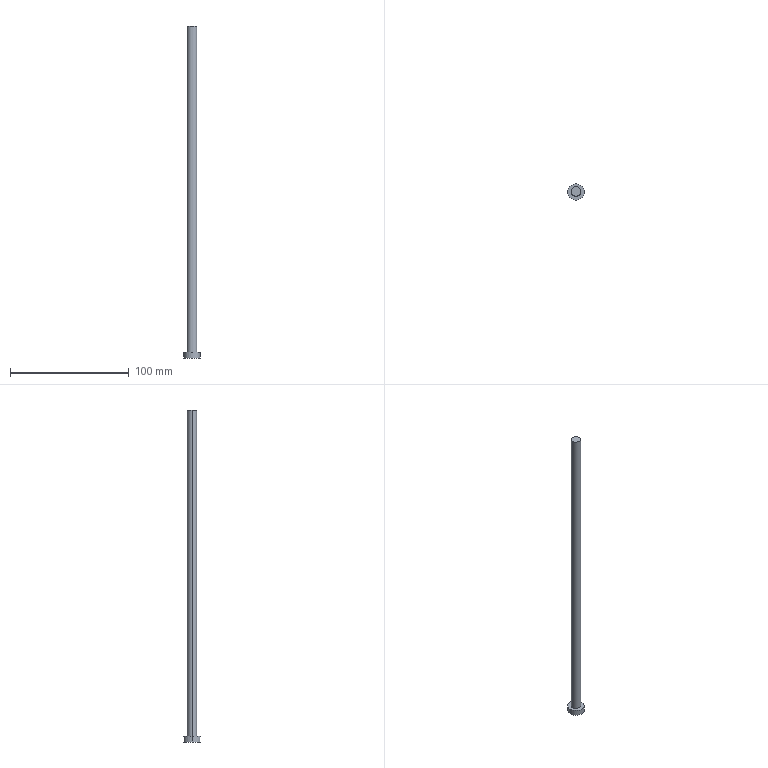Part | Creo | 1 solid | 7 faces | box 14 x 14 x 280.187 mm | volume 14602 mm3 | cylinder 4 | plane 3 | commonest cylinder face diameters 8 x2 14 x2
STEP:
#1=CARTESIAN_POINT('',(-171.,183.,44.687));
#2=VERTEX_POINT('',#1);
#3=CARTESIAN_POINT('',(-179.,183.,44.687));
#4=VERTEX_POINT('',#3);
#5=CARTESIAN_POINT('',(-175.,183.,44.687));
#6=DIRECTION('',(0.,0.,1.));
#7=DIRECTION('',(1.,0.,0.));
#8=AXIS2_PLACEMENT_3D('',#5,#6,#7);
#9=CIRCLE('',#8,4.);
#10=EDGE_CURVE('',#2,#4,#9,.T.);
#11=ORIENTED_EDGE('',*,*,#10,.T.);
#12=CARTESIAN_POINT('',(-179.,183.,-230.5));
#13=VERTEX_POINT('',#12);
#14=CARTESIAN_POINT('',(-179.,183.,44.687));
#15=DIRECTION('',(0.,0.,-1.));
#16=VECTOR('',#15,275.187);
#17=LINE('',#14,#16);
#18=EDGE_CURVE('',#4,#13,#17,.T.);
#19=ORIENTED_EDGE('',*,*,#18,.T.);
#20=CARTESIAN_POINT('',(-171.,183.,-230.5));
#21=VERTEX_POINT('',#20);
#22=CARTESIAN_POINT('',(-175.,183.,-230.5));
#23=DIRECTION('',(0.,0.,-1.));
#24=DIRECTION('',(-1.,0.,0.));
#25=AXIS2_PLACEMENT_3D('',#22,#23,#24);
#26=CIRCLE('',#25,4.);
#27=EDGE_CURVE('',#13,#21,#26,.T.);
#28=ORIENTED_EDGE('',*,*,#27,.T.);
#29=CARTESIAN_POINT('',(-171.,183.,44.687));
#30=DIRECTION('',(0.,0.,-1.));
#31=VECTOR('',#30,275.187);
#32=LINE('',#29,#31);
#33=EDGE_CURVE('',#2,#21,#32,.T.);
#34=ORIENTED_EDGE('',*,*,#33,.F.);
#35=EDGE_LOOP('',(#11,#19,#28,#34));
#36=FACE_OUTER_BOUND('',#35,.F.);
#37=CARTESIAN_POINT('',(-175.,183.,49.5));
#38=DIRECTION('',(0.,0.,-1.));
#39=DIRECTION('',(-1.,0.,0.));
#40=AXIS2_PLACEMENT_3D('',#37,#38,#39);
#41=CYLINDRICAL_SURFACE('',#40,4.);
#42=ADVANCED_FACE('',(#36),#41,.T.);
#43=ORIENTED_EDGE('',*,*,#10,.F.);
#44=CARTESIAN_POINT('',(-175.,183.,44.687));
#45=DIRECTION('',(0.,0.,1.));
#46=DIRECTION('',(-1.,0.,0.));
#47=AXIS2_PLACEMENT_3D('',#44,#45,#46);
#48=CIRCLE('',#47,4.);
#49=EDGE_CURVE('',#4,#2,#48,.T.);
#50=ORIENTED_EDGE('',*,*,#49,.F.);
#51=EDGE_LOOP('',(#43,#50));
#52=FACE_OUTER_BOUND('',#51,.F.);
#53=CARTESIAN_POINT('',(0.,0.,44.687));
#54=DIRECTION('',(0.,0.,1.));
#55=DIRECTION('',(1.,0.,0.));
#56=AXIS2_PLACEMENT_3D('',#53,#54,#55);
#57=PLANE('',#56);
#58=ADVANCED_FACE('',(#52),#57,.T.);
#59=ORIENTED_EDGE('',*,*,#49,.T.);
#60=ORIENTED_EDGE('',*,*,#33,.T.);
#61=CARTESIAN_POINT('',(-175.,183.,-230.5));
#62=DIRECTION('',(0.,0.,-1.));
#63=DIRECTION('',(1.,0.,0.));
#64=AXIS2_PLACEMENT_3D('',#61,#62,#63);
#65=CIRCLE('',#64,4.);
#66=EDGE_CURVE('',#21,#13,#65,.T.);
#67=ORIENTED_EDGE('',*,*,#66,.T.);
#68=ORIENTED_EDGE('',*,*,#18,.F.);
#69=EDGE_LOOP('',(#59,#60,#67,#68));
#70=FACE_OUTER_BOUND('',#69,.F.);
#71=CARTESIAN_POINT('',(-175.,183.,49.5));
#72=DIRECTION('',(0.,0.,-1.));
#73=DIRECTION('',(-1.,0.,0.));
#74=AXIS2_PLACEMENT_3D('',#71,#72,#73);
#75=CYLINDRICAL_SURFACE('',#74,4.);
#76=ADVANCED_FACE('',(#70),#75,.T.);
#77=CARTESIAN_POINT('',(-182.,183.,-230.5));
#78=VERTEX_POINT('',#77);
#79=CARTESIAN_POINT('',(-168.,183.,-230.5));
#80=VERTEX_POINT('',#79);
#81=CARTESIAN_POINT('',(-175.,183.,-230.5));
#82=DIRECTION('',(0.,0.,1.));
#83=DIRECTION('',(-1.,0.,0.));
#84=AXIS2_PLACEMENT_3D('',#81,#82,#83);
#85=CIRCLE('',#84,7.);
#86=EDGE_CURVE('',#78,#80,#85,.T.);
#87=ORIENTED_EDGE('',*,*,#86,.F.);
#88=CARTESIAN_POINT('',(-175.,183.,-230.5));
#89=DIRECTION('',(0.,0.,1.));
#90=DIRECTION('',(1.,0.,0.));
#91=AXIS2_PLACEMENT_3D('',#88,#89,#90);
#92=CIRCLE('',#91,7.);
#93=EDGE_CURVE('',#80,#78,#92,.T.);
#94=ORIENTED_EDGE('',*,*,#93,.F.);
#95=EDGE_LOOP('',(#87,#94));
#96=FACE_OUTER_BOUND('',#95,.F.);
#97=ORIENTED_EDGE('',*,*,#27,.F.);
#98=ORIENTED_EDGE('',*,*,#66,.F.);
#99=EDGE_LOOP('',(#97,#98));
#100=FACE_BOUND('',#99,.F.);
#101=CARTESIAN_POINT('',(-175.,183.,-230.5));
#102=DIRECTION('',(0.,0.,-1.));
#103=DIRECTION('',(-1.,0.,0.));
#104=AXIS2_PLACEMENT_3D('',#101,#102,#103);
#105=PLANE('',#104);
#106=ADVANCED_FACE('',(#96,#100),#105,.F.);
#107=CARTESIAN_POINT('',(-168.,183.,-235.5));
#108=VERTEX_POINT('',#107);
#109=CARTESIAN_POINT('',(-182.,183.,-235.5));
#110=VERTEX_POINT('',#109);
#111=CARTESIAN_POINT('',(-175.,183.,-235.5));
#112=DIRECTION('',(0.,0.,-1.));
#113=DIRECTION('',(1.,0.,0.));
#114=AXIS2_PLACEMENT_3D('',#111,#112,#113);
#115=CIRCLE('',#114,7.);
#116=EDGE_CURVE('',#108,#110,#115,.T.);
#117=ORIENTED_EDGE('',*,*,#116,.T.);
#118=CARTESIAN_POINT('',(-182.,183.,-230.5));
#119=DIRECTION('',(0.,0.,-1.));
#120=VECTOR('',#119,5.);
#121=LINE('',#118,#120);
#122=EDGE_CURVE('',#78,#110,#121,.T.);
#123=ORIENTED_EDGE('',*,*,#122,.F.);
#124=ORIENTED_EDGE('',*,*,#86,.T.);
#125=CARTESIAN_POINT('',(-168.,183.,-230.5));
#126=DIRECTION('',(0.,0.,-1.));
#127=VECTOR('',#126,5.);
#128=LINE('',#125,#127);
#129=EDGE_CURVE('',#80,#108,#128,.T.);
#130=ORIENTED_EDGE('',*,*,#129,.T.);
#131=EDGE_LOOP('',(#117,#123,#124,#130));
#132=FACE_OUTER_BOUND('',#131,.F.);
#133=CARTESIAN_POINT('',(-175.,183.,-245.913));
#134=DIRECTION('',(0.,0.,-1.));
#135=DIRECTION('',(-1.,0.,0.));
#136=AXIS2_PLACEMENT_3D('',#133,#134,#135);
#137=CYLINDRICAL_SURFACE('',#136,7.);
#138=ADVANCED_FACE('',(#132),#137,.T.);
#139=CARTESIAN_POINT('',(-175.,183.,-235.5));
#140=DIRECTION('',(0.,0.,-1.));
#141=DIRECTION('',(-1.,0.,0.));
#142=AXIS2_PLACEMENT_3D('',#139,#140,#141);
#143=CIRCLE('',#142,7.);
#144=EDGE_CURVE('',#110,#108,#143,.T.);
#145=ORIENTED_EDGE('',*,*,#144,.F.);
#146=ORIENTED_EDGE('',*,*,#116,.F.);
#147=EDGE_LOOP('',(#145,#146));
#148=FACE_OUTER_BOUND('',#147,.F.);
#149=CARTESIAN_POINT('',(-171.,183.,-235.5));
#150=DIRECTION('',(0.,0.,1.));
#151=DIRECTION('',(1.,0.,0.));
#152=AXIS2_PLACEMENT_3D('',#149,#150,#151);
#153=PLANE('',#152);
#154=ADVANCED_FACE('',(#148),#153,.F.);
#155=ORIENTED_EDGE('',*,*,#144,.T.);
#156=ORIENTED_EDGE('',*,*,#129,.F.);
#157=ORIENTED_EDGE('',*,*,#93,.T.);
#158=ORIENTED_EDGE('',*,*,#122,.T.);
#159=EDGE_LOOP('',(#155,#156,#157,#158));
#160=FACE_OUTER_BOUND('',#159,.F.);
#161=CARTESIAN_POINT('',(-175.,183.,-245.913));
#162=DIRECTION('',(0.,0.,-1.));
#163=DIRECTION('',(-1.,0.,0.));
#164=AXIS2_PLACEMENT_3D('',#161,#162,#163);
#165=CYLINDRICAL_SURFACE('',#164,7.);
#166=ADVANCED_FACE('',(#160),#165,.T.);
#167=CLOSED_SHELL('',(#42,#58,#76,#106,#138,#154,#166));
#168=MANIFOLD_SOLID_BREP('',#167);
#169=(LENGTH_UNIT()NAMED_UNIT(*)SI_UNIT(.MILLI.,.METRE.));
#170=UNCERTAINTY_MEASURE_WITH_UNIT(LENGTH_MEASURE(0.02809),#169,'','');
#171=(NAMED_UNIT(*)PLANE_ANGLE_UNIT()SI_UNIT($,.RADIAN.));
#172=PLANE_ANGLE_MEASURE_WITH_UNIT(PLANE_ANGLE_MEASURE(0.01745),#171);
#173=(CONVERSION_BASED_UNIT('DEGREE',#172)NAMED_UNIT(*)PLANE_ANGLE_UNIT());
#174=(NAMED_UNIT(*)SI_UNIT($,.STERADIAN.)SOLID_ANGLE_UNIT());
#175=(GEOMETRIC_REPRESENTATION_CONTEXT(3)GLOBAL_UNCERTAINTY_ASSIGNED_CONTEXT((#170))GLOBAL_UNIT_ASSIGNED_CONTEXT((#169,#173,#174))REPRESENTATION_CONTEXT('',''));
#176=ADVANCED_BREP_SHAPE_REPRESENTATION('',(#168),#175);